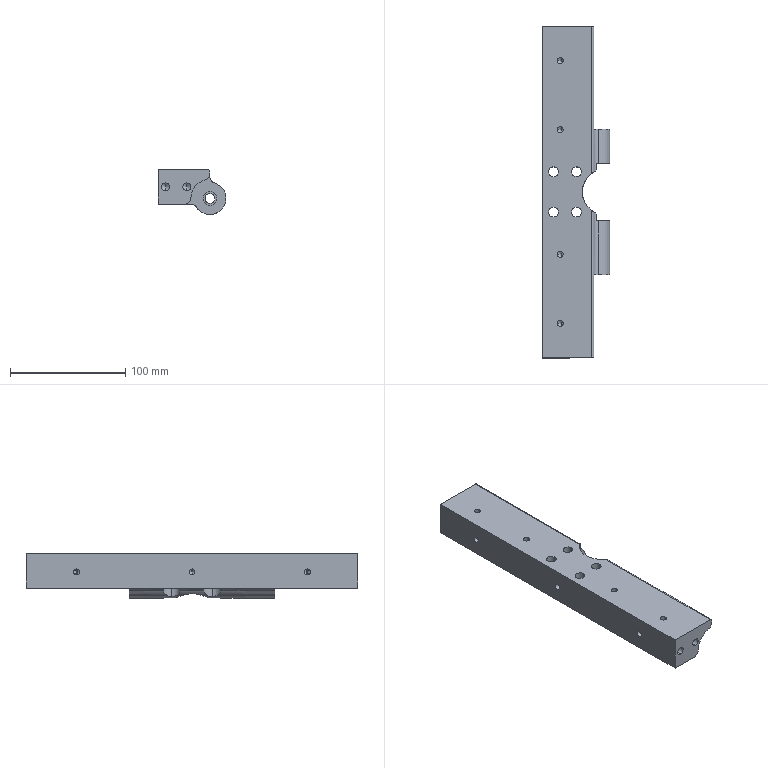Part | SolidWorks | features BaseBody 1 | 1 solid | 118 faces | box 59 x 288 x 39 mm | volume 333936 mm3 | cylinder 65 | cone 22 | plane 21 | spline 6 | sphere 4 | commonest cylinder face diameters 5.2 x14 10 x9 6.8 x8 8.4 x8 16 x8 6 x4